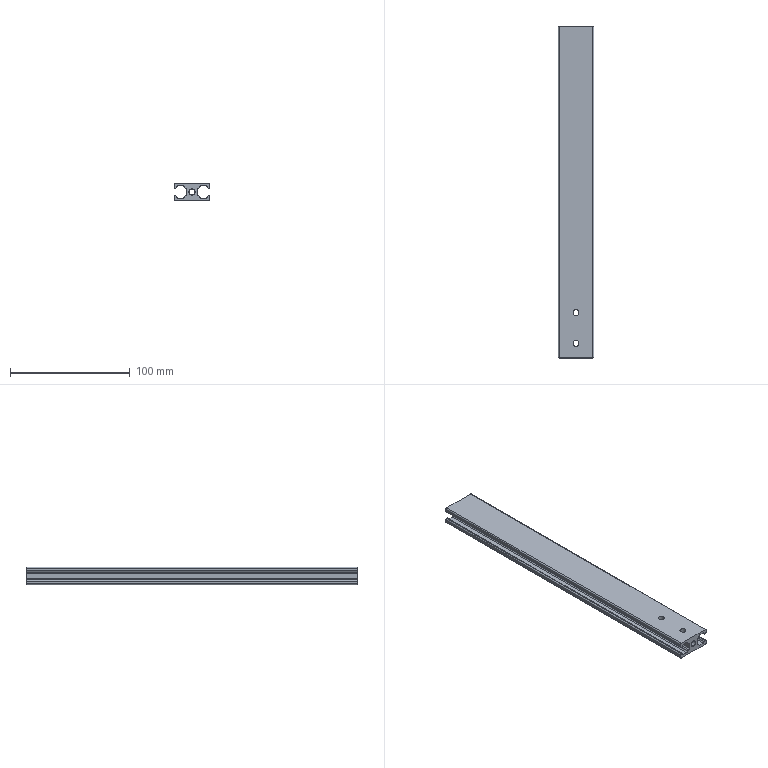Part | STEP file | GB1530T-6-30x15x275 | 1 solid | 60 faces | box 30 x 277 x 15 mm | volume 67010 mm3 | cylinder 38 | plane 22 | commonest cylinder face diameters 2 x28 5 x8 5.2 x2